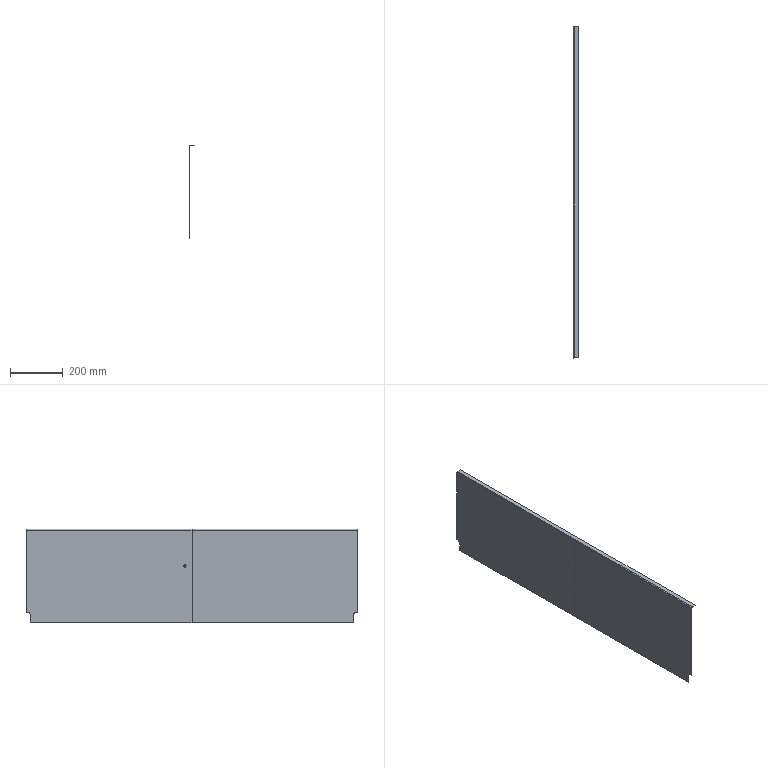Part | NX | features BREP 1 | 1 solid | 31 faces | box 20 x 1258 x 356.004 mm | volume 935299 mm3 | plane 21 | cylinder 10 | commonest cylinder face diameters 4 x4 8 x2 9 x2 20 x2
STEP:
#1=CARTESIAN_POINT('',(582.388,-0.001,379.004));
#2=VERTEX_POINT('',#1);
#3=CARTESIAN_POINT('',(582.388,629.17,379.004));
#4=VERTEX_POINT('',#3);
#5=CARTESIAN_POINT('',(582.388,0.,379.004));
#6=DIRECTION('',(0.,1.,0.));
#7=VECTOR('',#6,1000.);
#8=LINE('',#5,#7);
#9=EDGE_CURVE('',#2,#4,#8,.T.);
#10=ORIENTED_EDGE('',*,*,#9,.T.);
#11=CARTESIAN_POINT('',(598.388,629.17,379.004));
#12=VERTEX_POINT('',#11);
#13=CARTESIAN_POINT('',(590.388,629.17,379.004));
#14=DIRECTION('',(1.,0.,0.));
#15=VECTOR('',#14,1000.);
#16=LINE('',#13,#15);
#17=EDGE_CURVE('',#4,#12,#16,.T.);
#18=ORIENTED_EDGE('',*,*,#17,.T.);
#19=CARTESIAN_POINT('',(598.388,-629.17,379.004));
#20=VERTEX_POINT('',#19);
#21=CARTESIAN_POINT('',(598.388,0.,379.004));
#22=DIRECTION('',(0.,1.,0.));
#23=VECTOR('',#22,1000.);
#24=LINE('',#21,#23);
#25=EDGE_CURVE('',#20,#12,#24,.T.);
#26=ORIENTED_EDGE('',*,*,#25,.F.);
#27=CARTESIAN_POINT('',(582.388,-629.17,379.004));
#28=VERTEX_POINT('',#27);
#29=CARTESIAN_POINT('',(590.388,-629.17,379.004));
#30=DIRECTION('',(1.,0.,0.));
#31=VECTOR('',#30,1000.);
#32=LINE('',#29,#31);
#33=EDGE_CURVE('',#28,#20,#32,.T.);
#34=ORIENTED_EDGE('',*,*,#33,.F.);
#35=CARTESIAN_POINT('',(582.388,0.,379.004));
#36=DIRECTION('',(0.,-1.,0.));
#37=VECTOR('',#36,1000.);
#38=LINE('',#35,#37);
#39=EDGE_CURVE('',#2,#28,#38,.T.);
#40=ORIENTED_EDGE('',*,*,#39,.F.);
#41=EDGE_LOOP('',(#10,#18,#26,#34,#40));
#42=FACE_BOUND('',#41,.T.);
#43=CARTESIAN_POINT('',(578.388,-0.001,379.004));
#44=DIRECTION('',(0.,0.,-1.));
#45=DIRECTION('',(0.,1.,0.));
#46=AXIS2_PLACEMENT_3D('',#43,#44,#45);
#47=PLANE('',#46);
#48=ADVANCED_FACE('',(#42),#47,.T.);
#49=CARTESIAN_POINT('',(580.974,629.17,378.418));
#50=VERTEX_POINT('',#49);
#51=CARTESIAN_POINT('',(580.974,629.17,378.418));
#52=CARTESIAN_POINT('',(581.046,629.17,378.49));
#53=CARTESIAN_POINT('',(581.122,629.17,378.557));
#54=CARTESIAN_POINT('',(581.203,629.17,378.619));
#55=CARTESIAN_POINT('',(581.46,629.17,378.793));
#56=CARTESIAN_POINT('',(581.747,629.17,378.915));
#57=CARTESIAN_POINT('',(581.949,629.17,378.972));
#58=CARTESIAN_POINT('',(582.161,629.17,379.002));
#59=CARTESIAN_POINT('',(582.374,629.17,379.004));
#60=CARTESIAN_POINT('',(582.379,629.17,379.004));
#61=CARTESIAN_POINT('',(582.384,629.17,379.004));
#62=CARTESIAN_POINT('',(582.388,629.17,379.004));
#63=B_SPLINE_CURVE_WITH_KNOTS('',5,(#51,#52,#53,#54,#55,#56,#57,#58,#59,#60,#61,#62),.UNSPECIFIED.,.F.,.F.,(6,3,3,6),(2.221,2.939,4.409,4.443),.UNSPECIFIED.);
#64=EDGE_CURVE('',#50,#4,#63,.T.);
#65=ORIENTED_EDGE('',*,*,#64,.T.);
#66=ORIENTED_EDGE('',*,*,#9,.F.);
#67=CARTESIAN_POINT('',(580.974,-0.001,378.418));
#68=VERTEX_POINT('',#67);
#69=CARTESIAN_POINT('',(582.388,-0.001,379.004));
#70=CARTESIAN_POINT('',(581.996,-0.001,379.004));
#71=CARTESIAN_POINT('',(581.603,-0.001,378.901));
#72=CARTESIAN_POINT('',(581.252,-0.001,378.696));
#73=CARTESIAN_POINT('',(580.974,-0.001,378.418));
#74=B_SPLINE_CURVE_WITH_KNOTS('',4,(#69,#70,#71,#72,#73),.UNSPECIFIED.,.F.,.F.,(5,5),(-0.7854,0.7854),.UNSPECIFIED.);
#75=EDGE_CURVE('',#2,#68,#74,.T.);
#76=ORIENTED_EDGE('',*,*,#75,.T.);
#77=CARTESIAN_POINT('',(580.974,0.,378.418));
#78=DIRECTION('',(0.,1.,0.));
#79=VECTOR('',#78,1000.);
#80=LINE('',#77,#79);
#81=EDGE_CURVE('',#68,#50,#80,.T.);
#82=ORIENTED_EDGE('',*,*,#81,.T.);
#83=EDGE_LOOP('',(#65,#66,#76,#82));
#84=FACE_BOUND('',#83,.T.);
#85=CARTESIAN_POINT('',(582.388,0.,377.004));
#86=DIRECTION('',(0.,1.,0.));
#87=DIRECTION('',(-0.7071,0.,0.7071));
#88=AXIS2_PLACEMENT_3D('',#85,#86,#87);
#89=CYLINDRICAL_SURFACE('',#88,2.);
#90=ADVANCED_FACE('',(#84),#89,.F.);
#91=CARTESIAN_POINT('',(578.388,629.17,377.004));
#92=VERTEX_POINT('',#91);
#93=CARTESIAN_POINT('',(582.388,629.17,381.004));
#94=VERTEX_POINT('',#93);
#95=CARTESIAN_POINT('',(582.388,629.17,377.004));
#96=DIRECTION('',(0.,1.,0.));
#97=DIRECTION('',(1.,0.,0.));
#98=AXIS2_PLACEMENT_3D('',#95,#96,#97);
#99=CIRCLE('',#98,4.);
#100=EDGE_CURVE('',#92,#94,#99,.T.);
#101=ORIENTED_EDGE('',*,*,#100,.T.);
#102=CARTESIAN_POINT('',(582.388,629.17,380.004));
#103=DIRECTION('',(0.,0.,1.));
#104=VECTOR('',#103,1000.);
#105=LINE('',#102,#104);
#106=EDGE_CURVE('',#4,#94,#105,.T.);
#107=ORIENTED_EDGE('',*,*,#106,.F.);
#108=ORIENTED_EDGE('',*,*,#64,.F.);
#109=CARTESIAN_POINT('',(580.388,629.17,377.004));
#110=VERTEX_POINT('',#109);
#111=CARTESIAN_POINT('',(582.388,629.17,377.004));
#112=DIRECTION('',(0.,1.,0.));
#113=DIRECTION('',(1.,0.,0.));
#114=AXIS2_PLACEMENT_3D('',#111,#112,#113);
#115=CIRCLE('',#114,2.);
#116=EDGE_CURVE('',#110,#50,#115,.T.);
#117=ORIENTED_EDGE('',*,*,#116,.F.);
#118=CARTESIAN_POINT('',(579.388,629.17,377.004));
#119=DIRECTION('',(-1.,0.,0.));
#120=VECTOR('',#119,1000.);
#121=LINE('',#118,#120);
#122=EDGE_CURVE('',#110,#92,#121,.T.);
#123=ORIENTED_EDGE('',*,*,#122,.T.);
#124=EDGE_LOOP('',(#101,#107,#108,#117,#123));
#125=FACE_BOUND('',#124,.T.);
#126=CARTESIAN_POINT('',(582.388,629.17,381.004));
#127=DIRECTION('',(0.,-1.,0.));
#128=DIRECTION('',(-0.9239,0.,-0.3827));
#129=AXIS2_PLACEMENT_3D('',#126,#127,#128);
#130=PLANE('',#129);
#131=ADVANCED_FACE('',(#125),#130,.F.);
#132=CARTESIAN_POINT('',(598.388,629.17,381.004));
#133=VERTEX_POINT('',#132);
#134=CARTESIAN_POINT('',(598.388,629.17,380.004));
#135=DIRECTION('',(0.,0.,1.));
#136=VECTOR('',#135,1000.);
#137=LINE('',#134,#136);
#138=EDGE_CURVE('',#12,#133,#137,.T.);
#139=ORIENTED_EDGE('',*,*,#138,.F.);
#140=ORIENTED_EDGE('',*,*,#17,.F.);
#141=ORIENTED_EDGE('',*,*,#106,.T.);
#142=CARTESIAN_POINT('',(590.388,629.17,381.004));
#143=DIRECTION('',(1.,0.,0.));
#144=VECTOR('',#143,1000.);
#145=LINE('',#142,#144);
#146=EDGE_CURVE('',#94,#133,#145,.T.);
#147=ORIENTED_EDGE('',*,*,#146,.T.);
#148=EDGE_LOOP('',(#139,#140,#141,#147));
#149=FACE_BOUND('',#148,.T.);
#150=CARTESIAN_POINT('',(590.388,629.17,381.004));
#151=DIRECTION('',(0.,-1.,0.));
#152=DIRECTION('',(1.,0.,0.));
#153=AXIS2_PLACEMENT_3D('',#150,#151,#152);
#154=PLANE('',#153);
#155=ADVANCED_FACE('',(#149),#154,.F.);
#156=CARTESIAN_POINT('',(598.388,-629.17,381.004));
#157=VERTEX_POINT('',#156);
#158=CARTESIAN_POINT('',(598.388,-629.17,380.004));
#159=DIRECTION('',(0.,0.,1.));
#160=VECTOR('',#159,1000.);
#161=LINE('',#158,#160);
#162=EDGE_CURVE('',#20,#157,#161,.T.);
#163=ORIENTED_EDGE('',*,*,#162,.F.);
#164=ORIENTED_EDGE('',*,*,#25,.T.);
#165=ORIENTED_EDGE('',*,*,#138,.T.);
#166=CARTESIAN_POINT('',(598.388,0.,381.004));
#167=DIRECTION('',(0.,1.,0.));
#168=VECTOR('',#167,1000.);
#169=LINE('',#166,#168);
#170=EDGE_CURVE('',#157,#133,#169,.T.);
#171=ORIENTED_EDGE('',*,*,#170,.F.);
#172=EDGE_LOOP('',(#163,#164,#165,#171));
#173=FACE_BOUND('',#172,.T.);
#174=CARTESIAN_POINT('',(598.388,0.,381.004));
#175=DIRECTION('',(1.,0.,0.));
#176=DIRECTION('',(0.,1.,0.));
#177=AXIS2_PLACEMENT_3D('',#174,#175,#176);
#178=PLANE('',#177);
#179=ADVANCED_FACE('',(#173),#178,.T.);
#180=CARTESIAN_POINT('',(582.388,-629.17,381.004));
#181=VERTEX_POINT('',#180);
#182=CARTESIAN_POINT('',(582.388,-629.17,380.004));
#183=DIRECTION('',(0.,0.,1.));
#184=VECTOR('',#183,1000.);
#185=LINE('',#182,#184);
#186=EDGE_CURVE('',#28,#181,#185,.T.);
#187=ORIENTED_EDGE('',*,*,#186,.F.);
#188=ORIENTED_EDGE('',*,*,#33,.T.);
#189=ORIENTED_EDGE('',*,*,#162,.T.);
#190=CARTESIAN_POINT('',(590.388,-629.17,381.004));
#191=DIRECTION('',(1.,0.,0.));
#192=VECTOR('',#191,1000.);
#193=LINE('',#190,#192);
#194=EDGE_CURVE('',#181,#157,#193,.T.);
#195=ORIENTED_EDGE('',*,*,#194,.F.);
#196=EDGE_LOOP('',(#187,#188,#189,#195));
#197=FACE_BOUND('',#196,.T.);
#198=CARTESIAN_POINT('',(590.388,-629.17,381.004));
#199=DIRECTION('',(0.,-1.,0.));
#200=DIRECTION('',(1.,0.,0.));
#201=AXIS2_PLACEMENT_3D('',#198,#199,#200);
#202=PLANE('',#201);
#203=ADVANCED_FACE('',(#197),#202,.T.);
#204=ORIENTED_EDGE('',*,*,#75,.F.);
#205=ORIENTED_EDGE('',*,*,#39,.T.);
#206=CARTESIAN_POINT('',(580.974,-629.17,378.418));
#207=VERTEX_POINT('',#206);
#208=CARTESIAN_POINT('',(582.388,-629.17,377.004));
#209=DIRECTION('',(0.,-1.,0.));
#210=DIRECTION('',(1.,0.,0.));
#211=AXIS2_PLACEMENT_3D('',#208,#209,#210);
#212=CIRCLE('',#211,2.);
#213=EDGE_CURVE('',#28,#207,#212,.T.);
#214=ORIENTED_EDGE('',*,*,#213,.T.);
#215=CARTESIAN_POINT('',(580.974,0.,378.418));
#216=DIRECTION('',(0.,-1.,0.));
#217=VECTOR('',#216,1000.);
#218=LINE('',#215,#217);
#219=EDGE_CURVE('',#68,#207,#218,.T.);
#220=ORIENTED_EDGE('',*,*,#219,.F.);
#221=EDGE_LOOP('',(#204,#205,#214,#220));
#222=FACE_BOUND('',#221,.T.);
#223=CARTESIAN_POINT('',(582.388,0.,377.004));
#224=DIRECTION('',(0.,-1.,0.));
#225=DIRECTION('',(0.7071,0.,-0.7071));
#226=AXIS2_PLACEMENT_3D('',#223,#224,#225);
#227=CYLINDRICAL_SURFACE('',#226,2.);
#228=ADVANCED_FACE('',(#222),#227,.F.);
#229=CARTESIAN_POINT('',(580.388,-0.001,377.004));
#230=VERTEX_POINT('',#229);
#231=CARTESIAN_POINT('',(580.974,-0.001,378.418));
#232=CARTESIAN_POINT('',(580.696,-0.001,378.14));
#233=CARTESIAN_POINT('',(580.491,-0.001,377.789));
#234=CARTESIAN_POINT('',(580.388,-0.001,377.396));
#235=CARTESIAN_POINT('',(580.388,-0.001,377.004));
#236=B_SPLINE_CURVE_WITH_KNOTS('',4,(#231,#232,#233,#234,#235),.UNSPECIFIED.,.F.,.F.,(5,5),(-0.7854,0.7854),.UNSPECIFIED.);
#237=EDGE_CURVE('',#68,#230,#236,.T.);
#238=ORIENTED_EDGE('',*,*,#237,.T.);
#239=CARTESIAN_POINT('',(580.388,314.584,377.004));
#240=DIRECTION('',(0.,1.,0.));
#241=VECTOR('',#240,1000.);
#242=LINE('',#239,#241);
#243=EDGE_CURVE('',#230,#110,#242,.T.);
#244=ORIENTED_EDGE('',*,*,#243,.T.);
#245=ORIENTED_EDGE('',*,*,#116,.T.);
#246=ORIENTED_EDGE('',*,*,#81,.F.);
#247=EDGE_LOOP('',(#238,#244,#245,#246));
#248=FACE_BOUND('',#247,.T.);
#249=CARTESIAN_POINT('',(582.388,0.,377.004));
#250=DIRECTION('',(0.,1.,0.));
#251=DIRECTION('',(0.7071,0.,-0.7071));
#252=AXIS2_PLACEMENT_3D('',#249,#250,#251);
#253=CYLINDRICAL_SURFACE('',#252,2.);
#254=ADVANCED_FACE('',(#248),#253,.F.);
#255=CARTESIAN_POINT('',(578.388,27.072,245.997));
#256=VERTEX_POINT('',#255);
#257=CARTESIAN_POINT('',(580.388,27.072,245.997));
#258=VERTEX_POINT('',#257);
#259=CARTESIAN_POINT('',(580.388,27.072,245.997));
#260=CARTESIAN_POINT('',(578.388,27.072,245.997));
#261=B_SPLINE_CURVE_WITH_KNOTS('',1,(#259,#260),.UNSPECIFIED.,.F.,.F.,(2,2),(-2.,0.),.UNSPECIFIED.);
#262=EDGE_CURVE('',#256,#258,#261,.F.);
#263=ORIENTED_EDGE('',*,*,#262,.F.);
#264=CARTESIAN_POINT('',(578.388,27.072,236.997));
#265=VERTEX_POINT('',#264);
#266=CARTESIAN_POINT('',(578.388,27.072,236.997));
#267=CARTESIAN_POINT('',(578.388,28.252,236.997));
#268=CARTESIAN_POINT('',(578.388,30.594,237.969));
#269=CARTESIAN_POINT('',(578.388,32.061,241.496));
#270=CARTESIAN_POINT('',(578.388,30.595,245.022));
#271=CARTESIAN_POINT('',(578.388,28.255,245.997));
#272=CARTESIAN_POINT('',(578.388,27.072,245.997));
#273=B_SPLINE_CURVE_WITH_KNOTS('',3,(#266,#267,#268,#269,#270,#271,#272),.UNSPECIFIED.,.F.,.F.,(4,1,1,1,4),(0.,0.25,0.5,0.75,1.),.UNSPECIFIED.);
#274=EDGE_CURVE('',#256,#265,#273,.F.);
#275=ORIENTED_EDGE('',*,*,#274,.T.);
#276=CARTESIAN_POINT('',(580.388,27.072,236.997));
#277=VERTEX_POINT('',#276);
#278=CARTESIAN_POINT('',(580.388,27.072,236.997));
#279=CARTESIAN_POINT('',(578.388,27.072,236.997));
#280=B_SPLINE_CURVE_WITH_KNOTS('',1,(#278,#279),.UNSPECIFIED.,.F.,.F.,(2,2),(-2.,0.),.UNSPECIFIED.);
#281=EDGE_CURVE('',#265,#277,#280,.F.);
#282=ORIENTED_EDGE('',*,*,#281,.T.);
#283=CARTESIAN_POINT('',(580.388,27.072,245.997));
#284=CARTESIAN_POINT('',(580.388,28.254,245.997));
#285=CARTESIAN_POINT('',(580.388,30.596,245.022));
#286=CARTESIAN_POINT('',(580.388,32.061,241.496));
#287=CARTESIAN_POINT('',(580.388,30.594,237.969));
#288=CARTESIAN_POINT('',(580.388,28.254,236.997));
#289=CARTESIAN_POINT('',(580.388,27.072,236.997));
#290=B_SPLINE_CURVE_WITH_KNOTS('',3,(#283,#284,#285,#286,#287,#288,#289),.UNSPECIFIED.,.F.,.F.,(4,1,1,1,4),(0.,0.25,0.5,0.75,1.),.UNSPECIFIED.);
#291=EDGE_CURVE('',#258,#277,#290,.T.);
#292=ORIENTED_EDGE('',*,*,#291,.F.);
#293=EDGE_LOOP('',(#263,#275,#282,#292));
#294=FACE_BOUND('',#293,.T.);
#295=CARTESIAN_POINT('',(579.388,27.072,241.497));
#296=DIRECTION('',(1.,0.,0.));
#297=DIRECTION('',(0.,0.,-1.));
#298=AXIS2_PLACEMENT_3D('',#295,#296,#297);
#299=CYLINDRICAL_SURFACE('',#298,4.5);
#300=ADVANCED_FACE('',(#294),#299,.F.);
#301=CARTESIAN_POINT('',(580.388,27.072,236.997));
#302=CARTESIAN_POINT('',(580.388,25.891,236.997));
#303=CARTESIAN_POINT('',(580.388,23.549,237.97));
#304=CARTESIAN_POINT('',(580.388,22.083,241.497));
#305=CARTESIAN_POINT('',(580.388,23.551,245.024));
#306=CARTESIAN_POINT('',(580.388,25.89,245.997));
#307=CARTESIAN_POINT('',(580.388,27.072,245.997));
#308=B_SPLINE_CURVE_WITH_KNOTS('',3,(#301,#302,#303,#304,#305,#306,#307),.UNSPECIFIED.,.F.,.F.,(4,1,1,1,4),(0.,0.25,0.5,0.75,1.),.UNSPECIFIED.);
#309=EDGE_CURVE('',#277,#258,#308,.T.);
#310=ORIENTED_EDGE('',*,*,#309,.F.);
#311=ORIENTED_EDGE('',*,*,#281,.F.);
#312=CARTESIAN_POINT('',(578.388,27.072,245.997));
#313=CARTESIAN_POINT('',(578.388,25.893,245.997));
#314=CARTESIAN_POINT('',(578.388,23.551,245.025));
#315=CARTESIAN_POINT('',(578.388,22.083,241.498));
#316=CARTESIAN_POINT('',(578.388,23.549,237.971));
#317=CARTESIAN_POINT('',(578.388,25.889,236.997));
#318=CARTESIAN_POINT('',(578.388,27.072,236.997));
#319=B_SPLINE_CURVE_WITH_KNOTS('',3,(#312,#313,#314,#315,#316,#317,#318),.UNSPECIFIED.,.F.,.F.,(4,1,1,1,4),(0.,0.25,0.5,0.75,1.),.UNSPECIFIED.);
#320=EDGE_CURVE('',#265,#256,#319,.F.);
#321=ORIENTED_EDGE('',*,*,#320,.T.);
#322=ORIENTED_EDGE('',*,*,#262,.T.);
#323=EDGE_LOOP('',(#310,#311,#321,#322));
#324=FACE_BOUND('',#323,.T.);
#325=CARTESIAN_POINT('',(579.388,27.072,241.497));
#326=DIRECTION('',(1.,0.,0.));
#327=DIRECTION('',(0.,0.,-1.));
#328=AXIS2_PLACEMENT_3D('',#325,#326,#327);
#329=CYLINDRICAL_SURFACE('',#328,4.5);
#330=ADVANCED_FACE('',(#324),#329,.F.);
#331=CARTESIAN_POINT('',(578.388,622.5,65.));
#332=VERTEX_POINT('',#331);
#333=CARTESIAN_POINT('',(578.388,612.5,55.));
#334=VERTEX_POINT('',#333);
#335=CARTESIAN_POINT('',(578.388,622.5,65.));
#336=CARTESIAN_POINT('',(578.388,619.873,65.));
#337=CARTESIAN_POINT('',(578.388,614.673,62.829));
#338=CARTESIAN_POINT('',(578.388,612.5,57.629));
#339=CARTESIAN_POINT('',(578.388,612.5,55.));
#340=B_SPLINE_CURVE_WITH_KNOTS('',3,(#335,#336,#337,#338,#339),.UNSPECIFIED.,.F.,.F.,(4,1,4),(0.,0.5,1.),.UNSPECIFIED.);
#341=EDGE_CURVE('',#332,#334,#340,.T.);
#342=ORIENTED_EDGE('',*,*,#341,.F.);
#343=CARTESIAN_POINT('',(580.388,622.5,65.));
#344=VERTEX_POINT('',#343);
#345=CARTESIAN_POINT('',(579.388,622.5,65.));
#346=DIRECTION('',(-1.,0.,0.));
#347=VECTOR('',#346,1000.);
#348=LINE('',#345,#347);
#349=EDGE_CURVE('',#344,#332,#348,.T.);
#350=ORIENTED_EDGE('',*,*,#349,.F.);
#351=CARTESIAN_POINT('',(580.388,612.5,55.));
#352=VERTEX_POINT('',#351);
#353=CARTESIAN_POINT('',(580.388,612.5,55.));
#354=CARTESIAN_POINT('',(580.388,612.5,57.628));
#355=CARTESIAN_POINT('',(580.388,614.673,62.83));
#356=CARTESIAN_POINT('',(580.388,619.871,65.));
#357=CARTESIAN_POINT('',(580.388,622.5,65.));
#358=B_SPLINE_CURVE_WITH_KNOTS('',3,(#353,#354,#355,#356,#357),.UNSPECIFIED.,.F.,.F.,(4,1,4),(0.,0.5,1.),.UNSPECIFIED.);
#359=EDGE_CURVE('',#344,#352,#358,.F.);
#360=ORIENTED_EDGE('',*,*,#359,.T.);
#361=CARTESIAN_POINT('',(579.388,612.5,55.));
#362=DIRECTION('',(-1.,0.,0.));
#363=VECTOR('',#362,1000.);
#364=LINE('',#361,#363);
#365=EDGE_CURVE('',#352,#334,#364,.T.);
#366=ORIENTED_EDGE('',*,*,#365,.T.);
#367=EDGE_LOOP('',(#342,#350,#360,#366));
#368=FACE_BOUND('',#367,.T.);
#369=CARTESIAN_POINT('',(579.388,622.5,55.));
#370=DIRECTION('',(1.,0.,0.));
#371=DIRECTION('',(0.,1.,0.));
#372=AXIS2_PLACEMENT_3D('',#369,#370,#371);
#373=CYLINDRICAL_SURFACE('',#372,10.);
#374=ADVANCED_FACE('',(#368),#373,.F.);
#375=CARTESIAN_POINT('',(578.388,629.17,65.));
#376=VERTEX_POINT('',#375);
#377=CARTESIAN_POINT('',(578.388,629.17,65.));
#378=CARTESIAN_POINT('',(578.388,627.836,65.));
#379=CARTESIAN_POINT('',(578.388,626.502,65.));
#380=CARTESIAN_POINT('',(578.388,625.168,65.));
#381=CARTESIAN_POINT('',(578.388,623.834,65.));
#382=CARTESIAN_POINT('',(578.388,622.5,65.));
#383=B_SPLINE_CURVE_WITH_KNOTS('',5,(#377,#378,#379,#380,#381,#382),.UNSPECIFIED.,.F.,.F.,(6,6),(91.096,97.767),.UNSPECIFIED.);
#384=EDGE_CURVE('',#376,#332,#383,.T.);
#385=ORIENTED_EDGE('',*,*,#384,.F.);
#386=CARTESIAN_POINT('',(580.388,629.17,65.));
#387=VERTEX_POINT('',#386);
#388=CARTESIAN_POINT('',(579.388,629.17,65.));
#389=DIRECTION('',(-1.,0.,0.));
#390=VECTOR('',#389,1000.);
#391=LINE('',#388,#390);
#392=EDGE_CURVE('',#387,#376,#391,.T.);
#393=ORIENTED_EDGE('',*,*,#392,.F.);
#394=CARTESIAN_POINT('',(580.388,625.835,65.));
#395=DIRECTION('',(0.,-1.,0.));
#396=VECTOR('',#395,1000.);
#397=LINE('',#394,#396);
#398=EDGE_CURVE('',#387,#344,#397,.T.);
#399=ORIENTED_EDGE('',*,*,#398,.T.);
#400=ORIENTED_EDGE('',*,*,#349,.T.);
#401=EDGE_LOOP('',(#385,#393,#399,#400));
#402=FACE_BOUND('',#401,.T.);
#403=CARTESIAN_POINT('',(578.388,629.17,65.));
#404=DIRECTION('',(0.,0.,-1.));
#405=DIRECTION('',(0.,-1.,0.));
#406=AXIS2_PLACEMENT_3D('',#403,#404,#405);
#407=PLANE('',#406);
#408=ADVANCED_FACE('',(#402),#407,.T.);
#409=CARTESIAN_POINT('',(578.388,629.17,81.004));
#410=VERTEX_POINT('',#409);
#411=CARTESIAN_POINT('',(578.388,629.17,65.));
#412=CARTESIAN_POINT('',(578.388,629.17,65.4));
#413=CARTESIAN_POINT('',(578.388,629.17,65.8));
#414=CARTESIAN_POINT('',(578.388,629.17,66.2));
#415=CARTESIAN_POINT('',(578.388,629.17,69.401));
#416=CARTESIAN_POINT('',(578.388,629.17,72.601));
#417=CARTESIAN_POINT('',(578.388,629.17,75.402));
#418=CARTESIAN_POINT('',(578.388,629.17,78.203));
#419=CARTESIAN_POINT('',(578.388,629.17,81.004));
#420=B_SPLINE_CURVE_WITH_KNOTS('',5,(#411,#412,#413,#414,#415,#416,#417,#418,#419),.UNSPECIFIED.,.F.,.F.,(6,3,6),(604.597,606.597,620.601),.UNSPECIFIED.);
#421=EDGE_CURVE('',#376,#410,#420,.T.);
#422=ORIENTED_EDGE('',*,*,#421,.T.);
#423=CARTESIAN_POINT('',(580.388,629.17,81.004));
#424=VERTEX_POINT('',#423);
#425=CARTESIAN_POINT('',(579.388,629.17,81.004));
#426=DIRECTION('',(-1.,0.,0.));
#427=VECTOR('',#426,1000.);
#428=LINE('',#425,#427);
#429=EDGE_CURVE('',#424,#410,#428,.T.);
#430=ORIENTED_EDGE('',*,*,#429,.F.);
#431=CARTESIAN_POINT('',(580.388,629.17,73.002));
#432=DIRECTION('',(0.,0.,1.));
#433=VECTOR('',#432,1000.);
#434=LINE('',#431,#433);
#435=EDGE_CURVE('',#387,#424,#434,.T.);
#436=ORIENTED_EDGE('',*,*,#435,.F.);
#437=ORIENTED_EDGE('',*,*,#392,.T.);
#438=EDGE_LOOP('',(#422,#430,#436,#437));
#439=FACE_BOUND('',#438,.T.);
#440=CARTESIAN_POINT('',(578.388,629.17,65.));
#441=DIRECTION('',(0.,-1.,0.));
#442=DIRECTION('',(0.,0.,1.));
#443=AXIS2_PLACEMENT_3D('',#440,#441,#442);
#444=PLANE('',#443);
#445=ADVANCED_FACE('',(#439),#444,.F.);
#446=CARTESIAN_POINT('',(578.388,629.17,81.004));
#447=CARTESIAN_POINT('',(578.388,629.17,140.204));
#448=CARTESIAN_POINT('',(578.388,629.17,199.404));
#449=CARTESIAN_POINT('',(578.388,629.17,258.604));
#450=CARTESIAN_POINT('',(578.388,629.17,317.804));
#451=CARTESIAN_POINT('',(578.388,629.17,377.004));
#452=B_SPLINE_CURVE_WITH_KNOTS('',5,(#446,#447,#448,#449,#450,#451),.UNSPECIFIED.,.F.,.F.,(6,6),(620.601,916.601),.UNSPECIFIED.);
#453=EDGE_CURVE('',#410,#92,#452,.T.);
#454=ORIENTED_EDGE('',*,*,#453,.T.);
#455=ORIENTED_EDGE('',*,*,#122,.F.);
#456=CARTESIAN_POINT('',(580.388,629.17,229.004));
#457=DIRECTION('',(0.,0.,1.));
#458=VECTOR('',#457,1000.);
#459=LINE('',#456,#458);
#460=EDGE_CURVE('',#424,#110,#459,.T.);
#461=ORIENTED_EDGE('',*,*,#460,.F.);
#462=ORIENTED_EDGE('',*,*,#429,.T.);
#463=EDGE_LOOP('',(#454,#455,#461,#462));
#464=FACE_BOUND('',#463,.T.);
#465=CARTESIAN_POINT('',(578.388,629.17,81.004));
#466=DIRECTION('',(0.,-1.,0.));
#467=DIRECTION('',(0.,0.,1.));
#468=AXIS2_PLACEMENT_3D('',#465,#466,#467);
#469=PLANE('',#468);
#470=ADVANCED_FACE('',(#464),#469,.F.);
#471=CARTESIAN_POINT('',(578.388,-0.001,377.004));
#472=VERTEX_POINT('',#471);
#473=CARTESIAN_POINT('',(578.388,629.17,377.004));
#474=CARTESIAN_POINT('',(578.388,503.336,377.004));
#475=CARTESIAN_POINT('',(578.388,377.502,377.004));
#476=CARTESIAN_POINT('',(578.388,251.667,377.004));
#477=CARTESIAN_POINT('',(578.388,125.833,377.004));
#478=CARTESIAN_POINT('',(578.388,-0.001,377.004));
#479=B_SPLINE_CURVE_WITH_KNOTS('',5,(#473,#474,#475,#476,#477,#478),.UNSPECIFIED.,.F.,.F.,(6,6),(91.096,720.267),.UNSPECIFIED.);
#480=EDGE_CURVE('',#92,#472,#479,.T.);
#481=ORIENTED_EDGE('',*,*,#480,.T.);
#482=CARTESIAN_POINT('',(582.388,-0.001,381.004));
#483=VERTEX_POINT('',#482);
#484=CARTESIAN_POINT('',(582.388,-0.001,377.004));
#485=DIRECTION('',(0.,-1.,0.));
#486=DIRECTION('',(1.,0.,0.));
#487=AXIS2_PLACEMENT_3D('',#484,#485,#486);
#488=CIRCLE('',#487,4.);
#489=EDGE_CURVE('',#483,#472,#488,.T.);
#490=ORIENTED_EDGE('',*,*,#489,.F.);
#491=CARTESIAN_POINT('',(582.388,314.584,381.004));
#492=DIRECTION('',(0.,1.,0.));
#493=VECTOR('',#492,1000.);
#494=LINE('',#491,#493);
#495=EDGE_CURVE('',#483,#94,#494,.T.);
#496=ORIENTED_EDGE('',*,*,#495,.T.);
#497=ORIENTED_EDGE('',*,*,#100,.F.);
#498=EDGE_LOOP('',(#481,#490,#496,#497));
#499=FACE_BOUND('',#498,.T.);
#500=CARTESIAN_POINT('',(582.388,0.,377.004));
#501=DIRECTION('',(0.,1.,0.));
#502=DIRECTION('',(-1.,0.,0.));
#503=AXIS2_PLACEMENT_3D('',#500,#501,#502);
#504=CYLINDRICAL_SURFACE('',#503,4.);
#505=ADVANCED_FACE('',(#499),#504,.T.);
#506=CARTESIAN_POINT('',(582.388,0.,381.004));
#507=DIRECTION('',(0.,-1.,0.));
#508=VECTOR('',#507,1000.);
#509=LINE('',#506,#508);
#510=EDGE_CURVE('',#483,#181,#509,.T.);
#511=ORIENTED_EDGE('',*,*,#510,.T.);
#512=ORIENTED_EDGE('',*,*,#194,.T.);
#513=ORIENTED_EDGE('',*,*,#170,.T.);
#514=ORIENTED_EDGE('',*,*,#146,.F.);
#515=ORIENTED_EDGE('',*,*,#495,.F.);
#516=EDGE_LOOP('',(#511,#512,#513,#514,#515));
#517=FACE_BOUND('',#516,.T.);
#518=CARTESIAN_POINT('',(578.388,-0.001,381.004));
#519=DIRECTION('',(0.,0.,-1.));
#520=DIRECTION('',(0.,1.,0.));
#521=AXIS2_PLACEMENT_3D('',#518,#519,#520);
#522=PLANE('',#521);
#523=ADVANCED_FACE('',(#517),#522,.F.);
#524=CARTESIAN_POINT('',(578.388,-629.17,377.004));
#525=VERTEX_POINT('',#524);
#526=CARTESIAN_POINT('',(580.388,-629.17,377.004));
#527=VERTEX_POINT('',#526);
#528=CARTESIAN_POINT('',(579.388,-629.17,377.004));
#529=DIRECTION('',(1.,0.,0.));
#530=VECTOR('',#529,1000.);
#531=LINE('',#528,#530);
#532=EDGE_CURVE('',#525,#527,#531,.T.);
#533=ORIENTED_EDGE('',*,*,#532,.T.);
#534=CARTESIAN_POINT('',(582.388,-629.17,377.004));
#535=DIRECTION('',(0.,-1.,0.));
#536=DIRECTION('',(1.,0.,0.));
#537=AXIS2_PLACEMENT_3D('',#534,#535,#536);
#538=CIRCLE('',#537,2.);
#539=EDGE_CURVE('',#207,#527,#538,.T.);
#540=ORIENTED_EDGE('',*,*,#539,.F.);
#541=ORIENTED_EDGE('',*,*,#213,.F.);
#542=ORIENTED_EDGE('',*,*,#186,.T.);
#543=CARTESIAN_POINT('',(582.388,-629.17,377.004));
#544=DIRECTION('',(0.,-1.,0.));
#545=DIRECTION('',(1.,0.,0.));
#546=AXIS2_PLACEMENT_3D('',#543,#544,#545);
#547=CIRCLE('',#546,4.);
#548=EDGE_CURVE('',#181,#525,#547,.T.);
#549=ORIENTED_EDGE('',*,*,#548,.T.);
#550=EDGE_LOOP('',(#533,#540,#541,#542,#549));
#551=FACE_BOUND('',#550,.T.);
#552=CARTESIAN_POINT('',(582.388,-629.17,381.004));
#553=DIRECTION('',(0.,-1.,0.));
#554=DIRECTION('',(-0.9239,0.,-0.3827));
#555=AXIS2_PLACEMENT_3D('',#552,#553,#554);
#556=PLANE('',#555);
#557=ADVANCED_FACE('',(#551),#556,.T.);
#558=ORIENTED_EDGE('',*,*,#539,.T.);
#559=CARTESIAN_POINT('',(580.388,-314.586,377.004));
#560=DIRECTION('',(0.,-1.,0.));
#561=VECTOR('',#560,1000.);
#562=LINE('',#559,#561);
#563=EDGE_CURVE('',#230,#527,#562,.T.);
#564=ORIENTED_EDGE('',*,*,#563,.F.);
#565=ORIENTED_EDGE('',*,*,#237,.F.);
#566=ORIENTED_EDGE('',*,*,#219,.T.);
#567=EDGE_LOOP('',(#558,#564,#565,#566));
#568=FACE_BOUND('',#567,.T.);
#569=CARTESIAN_POINT('',(582.388,0.,377.004));
#570=DIRECTION('',(0.,-1.,0.));
#571=DIRECTION('',(-0.7071,0.,0.7071));
#572=AXIS2_PLACEMENT_3D('',#569,#570,#571);
#573=CYLINDRICAL_SURFACE('',#572,2.);
#574=ADVANCED_FACE('',(#568),#573,.F.);
#575=ORIENTED_EDGE('',*,*,#291,.T.);
#576=ORIENTED_EDGE('',*,*,#309,.T.);
#577=EDGE_LOOP('',(#575,#576));
#578=FACE_BOUND('',#577,.T.);
#579=ORIENTED_EDGE('',*,*,#359,.F.);
#580=ORIENTED_EDGE('',*,*,#398,.F.);
#581=ORIENTED_EDGE('',*,*,#435,.T.);
#582=ORIENTED_EDGE('',*,*,#460,.T.);
#583=ORIENTED_EDGE('',*,*,#243,.F.);
#584=CARTESIAN_POINT('',(580.388,-0.001,25.));
#585=VERTEX_POINT('',#584);
#586=CARTESIAN_POINT('',(580.388,-0.001,201.002));
#587=DIRECTION('',(0.,0.,1.));
#588=VECTOR('',#587,1000.);
#589=LINE('',#586,#588);
#590=EDGE_CURVE('',#585,#230,#589,.T.);
#591=ORIENTED_EDGE('',*,*,#590,.F.);
#592=CARTESIAN_POINT('',(580.388,612.5,25.));
#593=VERTEX_POINT('',#592);
#594=CARTESIAN_POINT('',(580.388,306.249,25.));
#595=DIRECTION('',(0.,-1.,0.));
#596=VECTOR('',#595,1000.);
#597=LINE('',#594,#596);
#598=EDGE_CURVE('',#593,#585,#597,.T.);
#599=ORIENTED_EDGE('',*,*,#598,.F.);
#600=CARTESIAN_POINT('',(580.388,612.5,40.));
#601=DIRECTION('',(0.,0.,1.));
#602=VECTOR('',#601,1000.);
#603=LINE('',#600,#602);
#604=EDGE_CURVE('',#593,#352,#603,.T.);
#605=ORIENTED_EDGE('',*,*,#604,.T.);
#606=EDGE_LOOP('',(#579,#580,#581,#582,#583,#591,#599,#605));
#607=FACE_BOUND('',#606,.T.);
#608=CARTESIAN_POINT('',(580.388,629.17,25.));
#609=DIRECTION('',(-1.,0.,0.));
#610=DIRECTION('',(0.,-1.,0.));
#611=AXIS2_PLACEMENT_3D('',#608,#609,#610);
#612=PLANE('',#611);
#613=ADVANCED_FACE('',(#578,#607),#612,.F.);
#614=CARTESIAN_POINT('',(578.388,612.5,25.));
#615=VERTEX_POINT('',#614);
#616=CARTESIAN_POINT('',(578.388,612.5,25.));
#617=CARTESIAN_POINT('',(578.388,612.5,31.));
#618=CARTESIAN_POINT('',(578.388,612.5,37.));
#619=CARTESIAN_POINT('',(578.388,612.5,43.));
#620=CARTESIAN_POINT('',(578.388,612.5,49.));
#621=CARTESIAN_POINT('',(578.388,612.5,55.));
#622=B_SPLINE_CURVE_WITH_KNOTS('',5,(#616,#617,#618,#619,#620,#621),.UNSPECIFIED.,.F.,.F.,(6,6),(564.597,594.597),.UNSPECIFIED.);
#623=EDGE_CURVE('',#615,#334,#622,.T.);
#624=ORIENTED_EDGE('',*,*,#623,.T.);
#625=ORIENTED_EDGE('',*,*,#365,.F.);
#626=ORIENTED_EDGE('',*,*,#604,.F.);
#627=CARTESIAN_POINT('',(579.388,612.5,25.));
#628=DIRECTION('',(-1.,0.,0.));
#629=VECTOR('',#628,1000.);
#630=LINE('',#627,#629);
#631=EDGE_CURVE('',#593,#615,#630,.T.);
#632=ORIENTED_EDGE('',*,*,#631,.T.);
#633=EDGE_LOOP('',(#624,#625,#626,#632));
#634=FACE_BOUND('',#633,.T.);
#635=CARTESIAN_POINT('',(578.388,612.5,25.));
#636=DIRECTION('',(0.,-1.,0.));
#637=DIRECTION('',(0.,0.,1.));
#638=AXIS2_PLACEMENT_3D('',#635,#636,#637);
#639=PLANE('',#638);
#640=ADVANCED_FACE('',(#634),#639,.F.);
#641=ORIENTED_EDGE('',*,*,#320,.F.);
#642=ORIENTED_EDGE('',*,*,#274,.F.);
#643=EDGE_LOOP('',(#641,#642));
#644=FACE_BOUND('',#643,.T.);
#645=ORIENTED_EDGE('',*,*,#623,.F.);
#646=CARTESIAN_POINT('',(578.388,-0.001,25.));
#647=VERTEX_POINT('',#646);
#648=CARTESIAN_POINT('',(578.388,306.249,25.));
#649=DIRECTION('',(0.,-1.,0.));
#650=VECTOR('',#649,1000.);
#651=LINE('',#648,#650);
#652=EDGE_CURVE('',#615,#647,#651,.T.);
#653=ORIENTED_EDGE('',*,*,#652,.T.);
#654=CARTESIAN_POINT('',(578.388,-0.001,25.));
#655=CARTESIAN_POINT('',(578.388,-0.001,33.4));
#656=CARTESIAN_POINT('',(578.388,-0.001,41.8));
#657=CARTESIAN_POINT('',(578.388,-0.001,50.2));
#658=CARTESIAN_POINT('',(578.388,-0.001,120.601));
#659=CARTESIAN_POINT('',(578.388,-0.001,191.001));
#660=CARTESIAN_POINT('',(578.388,-0.001,253.002));
#661=CARTESIAN_POINT('',(578.388,-0.001,315.003));
#662=CARTESIAN_POINT('',(578.388,-0.001,377.004));
#663=B_SPLINE_CURVE_WITH_KNOTS('',5,(#654,#655,#656,#657,#658,#659,#660,#661,#662),.UNSPECIFIED.,.F.,.F.,(6,3,6),(564.597,606.597,916.601),.UNSPECIFIED.);
#664=EDGE_CURVE('',#647,#472,#663,.T.);
#665=ORIENTED_EDGE('',*,*,#664,.T.);
#666=ORIENTED_EDGE('',*,*,#480,.F.);
#667=ORIENTED_EDGE('',*,*,#453,.F.);
#668=ORIENTED_EDGE('',*,*,#421,.F.);
#669=ORIENTED_EDGE('',*,*,#384,.T.);
#670=ORIENTED_EDGE('',*,*,#341,.T.);
#671=EDGE_LOOP('',(#645,#653,#665,#666,#667,#668,#669,#670));
#672=FACE_BOUND('',#671,.T.);
#673=CARTESIAN_POINT('',(578.388,360.677,370.55));
#674=DIRECTION('',(-1.,0.,0.));
#675=DIRECTION('',(0.,-1.,0.));
#676=AXIS2_PLACEMENT_3D('',#673,#674,#675);
#677=PLANE('',#676);
#678=ADVANCED_FACE('',(#644,#672),#677,.T.);
#679=CARTESIAN_POINT('',(578.388,-629.17,377.004));
#680=CARTESIAN_POINT('',(578.388,-503.336,377.004));
#681=CARTESIAN_POINT('',(578.388,-377.502,377.004));
#682=CARTESIAN_POINT('',(578.388,-251.669,377.004));
#683=CARTESIAN_POINT('',(578.388,-125.835,377.004));
#684=CARTESIAN_POINT('',(578.388,-0.001,377.004));
#685=B_SPLINE_CURVE_WITH_KNOTS('',5,(#679,#680,#681,#682,#683,#684),.UNSPECIFIED.,.F.,.F.,(6,6),(91.096,720.265),.UNSPECIFIED.);
#686=EDGE_CURVE('',#525,#472,#685,.T.);
#687=ORIENTED_EDGE('',*,*,#686,.F.);
#688=ORIENTED_EDGE('',*,*,#548,.F.);
#689=ORIENTED_EDGE('',*,*,#510,.F.);
#690=ORIENTED_EDGE('',*,*,#489,.T.);
#691=EDGE_LOOP('',(#687,#688,#689,#690));
#692=FACE_BOUND('',#691,.T.);
#693=CARTESIAN_POINT('',(582.388,0.,377.004));
#694=DIRECTION('',(0.,-1.,0.));
#695=DIRECTION('',(0.,0.,1.));
#696=AXIS2_PLACEMENT_3D('',#693,#694,#695);
#697=CYLINDRICAL_SURFACE('',#696,4.);
#698=ADVANCED_FACE('',(#692),#697,.T.);
#699=CARTESIAN_POINT('',(578.388,-629.17,81.004));
#700=VERTEX_POINT('',#699);
#701=CARTESIAN_POINT('',(580.388,-629.17,81.004));
#702=VERTEX_POINT('',#701);
#703=CARTESIAN_POINT('',(579.388,-629.17,81.004));
#704=DIRECTION('',(1.,0.,0.));
#705=VECTOR('',#704,1000.);
#706=LINE('',#703,#705);
#707=EDGE_CURVE('',#700,#702,#706,.T.);
#708=ORIENTED_EDGE('',*,*,#707,.T.);
#709=CARTESIAN_POINT('',(580.388,-629.17,229.004));
#710=DIRECTION('',(0.,0.,1.));
#711=VECTOR('',#710,1000.);
#712=LINE('',#709,#711);
#713=EDGE_CURVE('',#702,#527,#712,.T.);
#714=ORIENTED_EDGE('',*,*,#713,.T.);
#715=ORIENTED_EDGE('',*,*,#532,.F.);
#716=CARTESIAN_POINT('',(578.388,-629.17,81.004));
#717=CARTESIAN_POINT('',(578.388,-629.17,140.204));
#718=CARTESIAN_POINT('',(578.388,-629.17,199.404));
#719=CARTESIAN_POINT('',(578.388,-629.17,258.604));
#720=CARTESIAN_POINT('',(578.388,-629.17,317.804));
#721=CARTESIAN_POINT('',(578.388,-629.17,377.004));
#722=B_SPLINE_CURVE_WITH_KNOTS('',5,(#716,#717,#718,#719,#720,#721),.UNSPECIFIED.,.F.,.F.,(6,6),(620.601,916.601),.UNSPECIFIED.);
#723=EDGE_CURVE('',#700,#525,#722,.T.);
#724=ORIENTED_EDGE('',*,*,#723,.F.);
#725=EDGE_LOOP('',(#708,#714,#715,#724));
#726=FACE_BOUND('',#725,.T.);
#727=CARTESIAN_POINT('',(578.388,-629.17,81.004));
#728=DIRECTION('',(0.,1.,0.));
#729=DIRECTION('',(0.,0.,1.));
#730=AXIS2_PLACEMENT_3D('',#727,#728,#729);
#731=PLANE('',#730);
#732=ADVANCED_FACE('',(#726),#731,.F.);
#733=CARTESIAN_POINT('',(578.388,-629.17,65.));
#734=VERTEX_POINT('',#733);
#735=CARTESIAN_POINT('',(580.388,-629.17,65.));
#736=VERTEX_POINT('',#735);
#737=CARTESIAN_POINT('',(579.388,-629.17,65.));
#738=DIRECTION('',(1.,-0.000000001,0.));
#739=VECTOR('',#738,1000.);
#740=LINE('',#737,#739);
#741=EDGE_CURVE('',#734,#736,#740,.T.);
#742=ORIENTED_EDGE('',*,*,#741,.T.);
#743=CARTESIAN_POINT('',(580.388,-629.17,73.002));
#744=DIRECTION('',(0.,0.,1.));
#745=VECTOR('',#744,1000.);
#746=LINE('',#743,#745);
#747=EDGE_CURVE('',#736,#702,#746,.T.);
#748=ORIENTED_EDGE('',*,*,#747,.T.);
#749=ORIENTED_EDGE('',*,*,#707,.F.);
#750=CARTESIAN_POINT('',(578.388,-629.17,65.));
#751=CARTESIAN_POINT('',(578.388,-629.17,65.4));
#752=CARTESIAN_POINT('',(578.388,-629.17,65.8));
#753=CARTESIAN_POINT('',(578.388,-629.17,66.2));
#754=CARTESIAN_POINT('',(578.388,-629.17,69.401));
#755=CARTESIAN_POINT('',(578.388,-629.17,72.601));
#756=CARTESIAN_POINT('',(578.388,-629.17,75.402));
#757=CARTESIAN_POINT('',(578.388,-629.17,78.203));
#758=CARTESIAN_POINT('',(578.388,-629.17,81.004));
#759=B_SPLINE_CURVE_WITH_KNOTS('',5,(#750,#751,#752,#753,#754,#755,#756,#757,#758),.UNSPECIFIED.,.F.,.F.,(6,3,6),(604.597,606.597,620.601),.UNSPECIFIED.);
#760=EDGE_CURVE('',#734,#700,#759,.T.);
#761=ORIENTED_EDGE('',*,*,#760,.F.);
#762=EDGE_LOOP('',(#742,#748,#749,#761));
#763=FACE_BOUND('',#762,.T.);
#764=CARTESIAN_POINT('',(578.388,-629.17,65.));
#765=DIRECTION('',(0.,1.,0.));
#766=DIRECTION('',(0.,0.,1.));
#767=AXIS2_PLACEMENT_3D('',#764,#765,#766);
#768=PLANE('',#767);
#769=ADVANCED_FACE('',(#763),#768,.F.);
#770=CARTESIAN_POINT('',(578.388,-622.5,65.));
#771=VERTEX_POINT('',#770);
#772=CARTESIAN_POINT('',(580.388,-622.5,65.));
#773=VERTEX_POINT('',#772);
#774=CARTESIAN_POINT('',(578.388,-622.5,65.));
#775=CARTESIAN_POINT('',(580.388,-622.5,65.));
#776=B_SPLINE_CURVE_WITH_KNOTS('',1,(#774,#775),.UNSPECIFIED.,.F.,.F.,(2,2),(0.,2.),.UNSPECIFIED.);
#777=EDGE_CURVE('',#771,#773,#776,.T.);
#778=ORIENTED_EDGE('',*,*,#777,.T.);
#779=CARTESIAN_POINT('',(580.388,-625.835,65.));
#780=DIRECTION('',(0.,1.,0.));
#781=VECTOR('',#780,1000.);
#782=LINE('',#779,#781);
#783=EDGE_CURVE('',#736,#773,#782,.T.);
#784=ORIENTED_EDGE('',*,*,#783,.F.);
#785=ORIENTED_EDGE('',*,*,#741,.F.);
#786=CARTESIAN_POINT('',(578.388,-629.17,65.));
#787=CARTESIAN_POINT('',(578.388,-627.836,65.));
#788=CARTESIAN_POINT('',(578.388,-626.502,65.));
#789=CARTESIAN_POINT('',(578.388,-625.168,65.));
#790=CARTESIAN_POINT('',(578.388,-623.834,65.));
#791=CARTESIAN_POINT('',(578.388,-622.5,65.));
#792=B_SPLINE_CURVE_WITH_KNOTS('',5,(#786,#787,#788,#789,#790,#791),.UNSPECIFIED.,.F.,.F.,(6,6),(91.096,97.767),.UNSPECIFIED.);
#793=EDGE_CURVE('',#734,#771,#792,.T.);
#794=ORIENTED_EDGE('',*,*,#793,.T.);
#795=EDGE_LOOP('',(#778,#784,#785,#794));
#796=FACE_BOUND('',#795,.T.);
#797=CARTESIAN_POINT('',(578.388,-629.17,65.));
#798=DIRECTION('',(0.,0.,-1.));
#799=DIRECTION('',(0.,1.,0.));
#800=AXIS2_PLACEMENT_3D('',#797,#798,#799);
#801=PLANE('',#800);
#802=ADVANCED_FACE('',(#796),#801,.T.);
#803=CARTESIAN_POINT('',(578.388,-612.5,55.));
#804=VERTEX_POINT('',#803);
#805=CARTESIAN_POINT('',(580.388,-612.5,55.));
#806=VERTEX_POINT('',#805);
#807=CARTESIAN_POINT('',(579.388,-612.5,55.));
#808=DIRECTION('',(1.,0.,0.));
#809=VECTOR('',#808,1000.);
#810=LINE('',#807,#809);
#811=EDGE_CURVE('',#804,#806,#810,.T.);
#812=ORIENTED_EDGE('',*,*,#811,.T.);
#813=CARTESIAN_POINT('',(580.388,-622.5,65.));
#814=CARTESIAN_POINT('',(580.388,-619.873,65.));
#815=CARTESIAN_POINT('',(580.388,-614.673,62.829));
#816=CARTESIAN_POINT('',(580.388,-612.5,57.63));
#817=CARTESIAN_POINT('',(580.388,-612.5,55.));
#818=B_SPLINE_CURVE_WITH_KNOTS('',3,(#813,#814,#815,#816,#817),.UNSPECIFIED.,.F.,.F.,(4,1,4),(0.,0.5,1.),.UNSPECIFIED.);
#819=EDGE_CURVE('',#773,#806,#818,.T.);
#820=ORIENTED_EDGE('',*,*,#819,.F.);
#821=ORIENTED_EDGE('',*,*,#777,.F.);
#822=CARTESIAN_POINT('',(578.388,-612.5,55.));
#823=CARTESIAN_POINT('',(578.388,-612.5,57.628));
#824=CARTESIAN_POINT('',(578.388,-614.674,62.83));
#825=CARTESIAN_POINT('',(578.388,-619.871,65.));
#826=CARTESIAN_POINT('',(578.388,-622.5,65.));
#827=B_SPLINE_CURVE_WITH_KNOTS('',3,(#822,#823,#824,#825,#826),.UNSPECIFIED.,.F.,.F.,(4,1,4),(0.,0.5,1.),.UNSPECIFIED.);
#828=EDGE_CURVE('',#771,#804,#827,.F.);
#829=ORIENTED_EDGE('',*,*,#828,.T.);
#830=EDGE_LOOP('',(#812,#820,#821,#829));
#831=FACE_BOUND('',#830,.T.);
#832=CARTESIAN_POINT('',(579.388,-622.5,55.));
#833=DIRECTION('',(1.,0.,0.));
#834=DIRECTION('',(0.,1.,0.));
#835=AXIS2_PLACEMENT_3D('',#832,#833,#834);
#836=CYLINDRICAL_SURFACE('',#835,10.);
#837=ADVANCED_FACE('',(#831),#836,.F.);
#838=CARTESIAN_POINT('',(578.388,-612.5,25.));
#839=VERTEX_POINT('',#838);
#840=CARTESIAN_POINT('',(580.388,-612.5,25.));
#841=VERTEX_POINT('',#840);
#842=CARTESIAN_POINT('',(579.388,-612.5,25.));
#843=DIRECTION('',(1.,0.,0.));
#844=VECTOR('',#843,1000.);
#845=LINE('',#842,#844);
#846=EDGE_CURVE('',#839,#841,#845,.T.);
#847=ORIENTED_EDGE('',*,*,#846,.T.);
#848=CARTESIAN_POINT('',(580.388,-612.5,40.));
#849=DIRECTION('',(0.,0.,1.));
#850=VECTOR('',#849,1000.);
#851=LINE('',#848,#850);
#852=EDGE_CURVE('',#841,#806,#851,.T.);
#853=ORIENTED_EDGE('',*,*,#852,.T.);
#854=ORIENTED_EDGE('',*,*,#811,.F.);
#855=CARTESIAN_POINT('',(578.388,-612.5,25.));
#856=CARTESIAN_POINT('',(578.388,-612.5,31.));
#857=CARTESIAN_POINT('',(578.388,-612.5,37.));
#858=CARTESIAN_POINT('',(578.388,-612.5,43.));
#859=CARTESIAN_POINT('',(578.388,-612.5,49.));
#860=CARTESIAN_POINT('',(578.388,-612.5,55.));
#861=B_SPLINE_CURVE_WITH_KNOTS('',5,(#855,#856,#857,#858,#859,#860),.UNSPECIFIED.,.F.,.F.,(6,6),(564.597,594.597),.UNSPECIFIED.);
#862=EDGE_CURVE('',#839,#804,#861,.T.);
#863=ORIENTED_EDGE('',*,*,#862,.F.);
#864=EDGE_LOOP('',(#847,#853,#854,#863));
#865=FACE_BOUND('',#864,.T.);
#866=CARTESIAN_POINT('',(578.388,-612.5,25.));
#867=DIRECTION('',(0.,1.,0.));
#868=DIRECTION('',(0.,0.,1.));
#869=AXIS2_PLACEMENT_3D('',#866,#867,#868);
#870=PLANE('',#869);
#871=ADVANCED_FACE('',(#865),#870,.F.);
#872=CARTESIAN_POINT('',(580.388,-306.25,25.));
#873=DIRECTION('',(0.,1.,0.));
#874=VECTOR('',#873,1000.);
#875=LINE('',#872,#874);
#876=EDGE_CURVE('',#841,#585,#875,.T.);
#877=ORIENTED_EDGE('',*,*,#876,.T.);
#878=ORIENTED_EDGE('',*,*,#590,.T.);
#879=ORIENTED_EDGE('',*,*,#563,.T.);
#880=ORIENTED_EDGE('',*,*,#713,.F.);
#881=ORIENTED_EDGE('',*,*,#747,.F.);
#882=ORIENTED_EDGE('',*,*,#783,.T.);
#883=ORIENTED_EDGE('',*,*,#819,.T.);
#884=ORIENTED_EDGE('',*,*,#852,.F.);
#885=EDGE_LOOP('',(#877,#878,#879,#880,#881,#882,#883,#884));
#886=FACE_BOUND('',#885,.T.);
#887=CARTESIAN_POINT('',(580.388,-629.17,25.));
#888=DIRECTION('',(1.,0.,0.));
#889=DIRECTION('',(0.,1.,0.));
#890=AXIS2_PLACEMENT_3D('',#887,#888,#889);
#891=PLANE('',#890);
#892=ADVANCED_FACE('',(#886),#891,.T.);
#893=ORIENTED_EDGE('',*,*,#652,.F.);
#894=ORIENTED_EDGE('',*,*,#631,.F.);
#895=ORIENTED_EDGE('',*,*,#598,.T.);
#896=CARTESIAN_POINT('',(579.388,-0.001,25.));
#897=DIRECTION('',(1.,-0.000000001,0.));
#898=VECTOR('',#897,1000.);
#899=LINE('',#896,#898);
#900=EDGE_CURVE('',#647,#585,#899,.T.);
#901=ORIENTED_EDGE('',*,*,#900,.F.);
#902=EDGE_LOOP('',(#893,#894,#895,#901));
#903=FACE_BOUND('',#902,.T.);
#904=CARTESIAN_POINT('',(578.388,612.5,25.));
#905=DIRECTION('',(0.,0.,-1.));
#906=DIRECTION('',(0.,-1.,0.));
#907=AXIS2_PLACEMENT_3D('',#904,#905,#906);
#908=PLANE('',#907);
#909=ADVANCED_FACE('',(#903),#908,.T.);
#910=ORIENTED_EDGE('',*,*,#862,.T.);
#911=ORIENTED_EDGE('',*,*,#828,.F.);
#912=ORIENTED_EDGE('',*,*,#793,.F.);
#913=ORIENTED_EDGE('',*,*,#760,.T.);
#914=ORIENTED_EDGE('',*,*,#723,.T.);
#915=ORIENTED_EDGE('',*,*,#686,.T.);
#916=ORIENTED_EDGE('',*,*,#664,.F.);
#917=CARTESIAN_POINT('',(578.388,-306.25,25.));
#918=DIRECTION('',(0.,1.,0.));
#919=VECTOR('',#918,1000.);
#920=LINE('',#917,#919);
#921=EDGE_CURVE('',#839,#647,#920,.T.);
#922=ORIENTED_EDGE('',*,*,#921,.F.);
#923=EDGE_LOOP('',(#910,#911,#912,#913,#914,#915,#916,#922));
#924=FACE_BOUND('',#923,.T.);
#925=CARTESIAN_POINT('',(578.388,-360.677,370.55));
#926=DIRECTION('',(1.,0.,0.));
#927=DIRECTION('',(0.,1.,0.));
#928=AXIS2_PLACEMENT_3D('',#925,#926,#927);
#929=PLANE('',#928);
#930=ADVANCED_FACE('',(#924),#929,.F.);
#931=ORIENTED_EDGE('',*,*,#921,.T.);
#932=ORIENTED_EDGE('',*,*,#900,.T.);
#933=ORIENTED_EDGE('',*,*,#876,.F.);
#934=ORIENTED_EDGE('',*,*,#846,.F.);
#935=EDGE_LOOP('',(#931,#932,#933,#934));
#936=FACE_BOUND('',#935,.T.);
#937=CARTESIAN_POINT('',(578.388,-612.5,25.));
#938=DIRECTION('',(0.,0.,-1.));
#939=DIRECTION('',(0.,1.,0.));
#940=AXIS2_PLACEMENT_3D('',#937,#938,#939);
#941=PLANE('',#940);
#942=ADVANCED_FACE('',(#936),#941,.T.);
#943=CLOSED_SHELL('',(#48,#90,#131,#155,#179,#203,#228,#254,#300,#330,#374,#408,#445,#470,#505,#523,#557,#574,#613,#640,#678,#698,#732,#769,#802,#837,#871,#892,#909,#930,#942));
#944=MANIFOLD_SOLID_BREP('',#943);
#945=(LENGTH_UNIT()NAMED_UNIT(*)SI_UNIT(.MILLI.,.METRE.));
#946=UNCERTAINTY_MEASURE_WITH_UNIT(LENGTH_MEASURE(0.0508),#945,'','');
#947=(NAMED_UNIT(*)PLANE_ANGLE_UNIT()SI_UNIT($,.RADIAN.));
#948=(NAMED_UNIT(*)SI_UNIT($,.STERADIAN.)SOLID_ANGLE_UNIT());
#949=(GEOMETRIC_REPRESENTATION_CONTEXT(3)GLOBAL_UNCERTAINTY_ASSIGNED_CONTEXT((#946))GLOBAL_UNIT_ASSIGNED_CONTEXT((#945,#947,#948))REPRESENTATION_CONTEXT('',''));
#950=ADVANCED_BREP_SHAPE_REPRESENTATION('',(#944),#949);